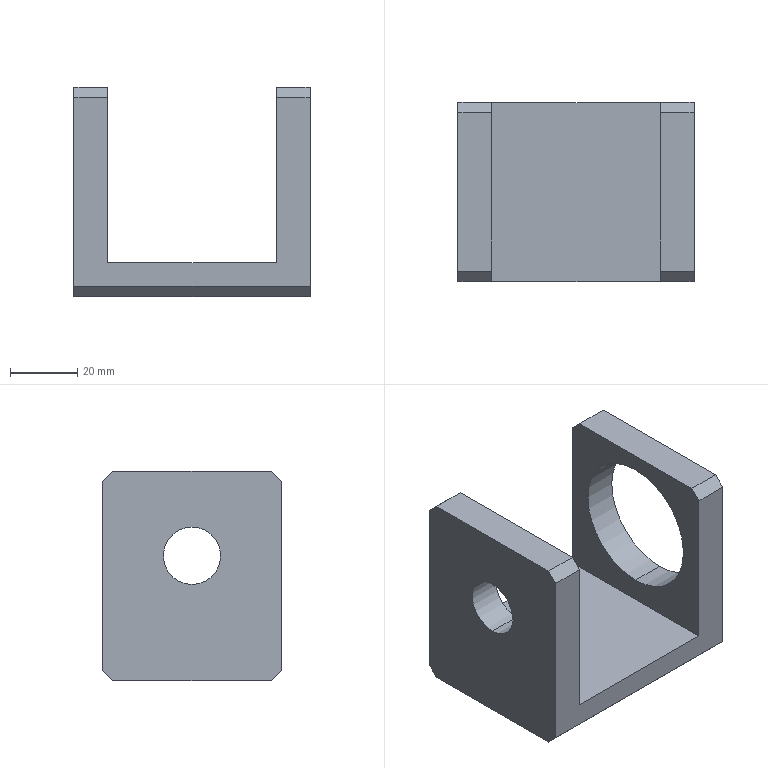Part | SolidWorks | features ICE 4, Chamfer 3, 3DProfileFeature 1, Extrusion 1, HoleWzd 1 | 1 solid | 20 faces | box 70 x 53 x 62 mm | volume 76574 mm3 | plane 16 | cylinder 4 | commonest cylinder face diameters 17 x2 40 x2
STEP:
#1=CARTESIAN_POINT('',(60.,0.,-5.));
#2=VERTEX_POINT('',#1);
#3=CARTESIAN_POINT('',(60.,0.,-45.));
#4=VERTEX_POINT('',#3);
#5=CARTESIAN_POINT('',(60.,0.,-25.));
#6=DIRECTION('',(1.,0.,0.));
#7=DIRECTION('',(0.,0.,1.));
#8=AXIS2_PLACEMENT_3D('',#5,#6,#7);
#9=CIRCLE('',#8,20.);
#10=EDGE_CURVE('',#2,#4,#9,.T.);
#11=ORIENTED_EDGE('',*,*,#10,.T.);
#12=CARTESIAN_POINT('',(50.,0.,-45.));
#13=VERTEX_POINT('',#12);
#14=CARTESIAN_POINT('',(60.001,0.,-45.));
#15=DIRECTION('',(-1.,0.,0.));
#16=VECTOR('',#15,1000.);
#17=LINE('',#14,#16);
#18=EDGE_CURVE('',#4,#13,#17,.T.);
#19=ORIENTED_EDGE('',*,*,#18,.T.);
#20=CARTESIAN_POINT('',(50.,0.,-5.));
#21=VERTEX_POINT('',#20);
#22=CARTESIAN_POINT('',(50.,0.,-25.));
#23=DIRECTION('',(-1.,0.,0.));
#24=DIRECTION('',(0.,0.,1.));
#25=AXIS2_PLACEMENT_3D('',#22,#23,#24);
#26=CIRCLE('',#25,20.);
#27=EDGE_CURVE('',#13,#21,#26,.T.);
#28=ORIENTED_EDGE('',*,*,#27,.T.);
#29=CARTESIAN_POINT('',(60.001,0.,-5.));
#30=DIRECTION('',(-1.,0.,0.));
#31=VECTOR('',#30,1000.);
#32=LINE('',#29,#31);
#33=EDGE_CURVE('',#2,#21,#32,.T.);
#34=ORIENTED_EDGE('',*,*,#33,.F.);
#35=EDGE_LOOP('',(#11,#19,#28,#34));
#36=FACE_OUTER_BOUND('',#35,.T.);
#37=CARTESIAN_POINT('',(60.001,0.,-25.));
#38=DIRECTION('',(-1.,0.,0.));
#39=DIRECTION('',(0.,0.,1.));
#40=AXIS2_PLACEMENT_3D('',#37,#38,#39);
#41=CYLINDRICAL_SURFACE('',#40,20.);
#42=ADVANCED_FACE('',(#36),#41,.F.);
#43=CARTESIAN_POINT('',(0.,0.,-16.5));
#44=VERTEX_POINT('',#43);
#45=CARTESIAN_POINT('',(0.,0.,-33.5));
#46=VERTEX_POINT('',#45);
#47=CARTESIAN_POINT('',(0.,0.,-25.));
#48=DIRECTION('',(1.,0.,0.));
#49=DIRECTION('',(0.,0.,1.));
#50=AXIS2_PLACEMENT_3D('',#47,#48,#49);
#51=CIRCLE('',#50,8.5);
#52=EDGE_CURVE('',#44,#46,#51,.T.);
#53=ORIENTED_EDGE('',*,*,#52,.T.);
#54=CARTESIAN_POINT('',(-10.,0.,-33.5));
#55=VERTEX_POINT('',#54);
#56=CARTESIAN_POINT('',(60.001,0.,-33.5));
#57=DIRECTION('',(-1.,0.,0.));
#58=VECTOR('',#57,1000.);
#59=LINE('',#56,#58);
#60=EDGE_CURVE('',#46,#55,#59,.T.);
#61=ORIENTED_EDGE('',*,*,#60,.T.);
#62=CARTESIAN_POINT('',(-10.,0.,-16.5));
#63=VERTEX_POINT('',#62);
#64=CARTESIAN_POINT('',(-10.,0.,-25.));
#65=DIRECTION('',(-1.,0.,0.));
#66=DIRECTION('',(0.,0.,1.));
#67=AXIS2_PLACEMENT_3D('',#64,#65,#66);
#68=CIRCLE('',#67,8.5);
#69=EDGE_CURVE('',#55,#63,#68,.T.);
#70=ORIENTED_EDGE('',*,*,#69,.T.);
#71=CARTESIAN_POINT('',(60.001,0.,-16.5));
#72=DIRECTION('',(-1.,0.,0.));
#73=VECTOR('',#72,1000.);
#74=LINE('',#71,#73);
#75=EDGE_CURVE('',#44,#63,#74,.T.);
#76=ORIENTED_EDGE('',*,*,#75,.F.);
#77=EDGE_LOOP('',(#53,#61,#70,#76));
#78=FACE_OUTER_BOUND('',#77,.T.);
#79=CARTESIAN_POINT('',(60.001,0.,-25.));
#80=DIRECTION('',(-1.,0.,0.));
#81=DIRECTION('',(0.,0.,1.));
#82=AXIS2_PLACEMENT_3D('',#79,#80,#81);
#83=CYLINDRICAL_SURFACE('',#82,8.5);
#84=ADVANCED_FACE('',(#78),#83,.F.);
#85=CARTESIAN_POINT('',(-10.,23.5,0.));
#86=VERTEX_POINT('',#85);
#87=CARTESIAN_POINT('',(-10.,-23.5,0.));
#88=VERTEX_POINT('',#87);
#89=CARTESIAN_POINT('',(-10.,26.5,0.));
#90=DIRECTION('',(0.,-1.,0.));
#91=VECTOR('',#90,1000.);
#92=LINE('',#89,#91);
#93=EDGE_CURVE('',#86,#88,#92,.T.);
#94=ORIENTED_EDGE('',*,*,#93,.T.);
#95=CARTESIAN_POINT('',(0.,-23.5,0.));
#96=VERTEX_POINT('',#95);
#97=CARTESIAN_POINT('',(0.,-23.5,0.));
#98=DIRECTION('',(1.,0.,0.));
#99=VECTOR('',#98,1000.);
#100=LINE('',#97,#99);
#101=EDGE_CURVE('',#88,#96,#100,.T.);
#102=ORIENTED_EDGE('',*,*,#101,.T.);
#103=CARTESIAN_POINT('',(0.,23.5,0.));
#104=VERTEX_POINT('',#103);
#105=CARTESIAN_POINT('',(0.,26.5,0.));
#106=DIRECTION('',(0.,-1.,0.));
#107=VECTOR('',#106,1000.);
#108=LINE('',#105,#107);
#109=EDGE_CURVE('',#104,#96,#108,.T.);
#110=ORIENTED_EDGE('',*,*,#109,.F.);
#111=CARTESIAN_POINT('',(0.,23.5,0.));
#112=DIRECTION('',(-1.,0.,0.));
#113=VECTOR('',#112,1000.);
#114=LINE('',#111,#113);
#115=EDGE_CURVE('',#104,#86,#114,.T.);
#116=ORIENTED_EDGE('',*,*,#115,.T.);
#117=EDGE_LOOP('',(#94,#102,#110,#116));
#118=FACE_OUTER_BOUND('',#117,.T.);
#119=CARTESIAN_POINT('',(0.,26.5,0.));
#120=DIRECTION('',(0.,0.,-1.));
#121=DIRECTION('',(-1.,0.,0.));
#122=AXIS2_PLACEMENT_3D('',#119,#120,#121);
#123=PLANE('',#122);
#124=ADVANCED_FACE('',(#118),#123,.F.);
#125=ORIENTED_EDGE('',*,*,#52,.F.);
#126=CARTESIAN_POINT('',(0.,0.,-25.));
#127=DIRECTION('',(1.,0.,0.));
#128=DIRECTION('',(0.,0.,1.));
#129=AXIS2_PLACEMENT_3D('',#126,#127,#128);
#130=CIRCLE('',#129,8.5);
#131=EDGE_CURVE('',#46,#44,#130,.T.);
#132=ORIENTED_EDGE('',*,*,#131,.F.);
#133=EDGE_LOOP('',(#125,#132));
#134=FACE_BOUND('',#133,.T.);
#135=ORIENTED_EDGE('',*,*,#109,.T.);
#136=CARTESIAN_POINT('',(0.,-26.5,-3.));
#137=VERTEX_POINT('',#136);
#138=CARTESIAN_POINT('',(0.,-23.5,0.));
#139=DIRECTION('',(0.,-0.7071,-0.7071));
#140=VECTOR('',#139,1000.);
#141=LINE('',#138,#140);
#142=EDGE_CURVE('',#96,#137,#141,.T.);
#143=ORIENTED_EDGE('',*,*,#142,.T.);
#144=CARTESIAN_POINT('',(0.,-26.5,-52.));
#145=VERTEX_POINT('',#144);
#146=CARTESIAN_POINT('',(0.,-26.5,0.));
#147=DIRECTION('',(0.,0.,-1.));
#148=VECTOR('',#147,1000.);
#149=LINE('',#146,#148);
#150=EDGE_CURVE('',#137,#145,#149,.T.);
#151=ORIENTED_EDGE('',*,*,#150,.T.);
#152=CARTESIAN_POINT('',(0.,26.5,-52.));
#153=VERTEX_POINT('',#152);
#154=CARTESIAN_POINT('',(0.,26.5,-52.));
#155=DIRECTION('',(0.,-1.,0.));
#156=VECTOR('',#155,1000.);
#157=LINE('',#154,#156);
#158=EDGE_CURVE('',#153,#145,#157,.T.);
#159=ORIENTED_EDGE('',*,*,#158,.F.);
#160=CARTESIAN_POINT('',(0.,26.5,-3.));
#161=VERTEX_POINT('',#160);
#162=CARTESIAN_POINT('',(0.,26.5,0.));
#163=DIRECTION('',(0.,0.,-1.));
#164=VECTOR('',#163,1000.);
#165=LINE('',#162,#164);
#166=EDGE_CURVE('',#161,#153,#165,.T.);
#167=ORIENTED_EDGE('',*,*,#166,.F.);
#168=CARTESIAN_POINT('',(0.,26.5,-3.));
#169=DIRECTION('',(0.,-0.7071,0.7071));
#170=VECTOR('',#169,1000.);
#171=LINE('',#168,#170);
#172=EDGE_CURVE('',#161,#104,#171,.T.);
#173=ORIENTED_EDGE('',*,*,#172,.T.);
#174=EDGE_LOOP('',(#135,#143,#151,#159,#167,#173));
#175=FACE_OUTER_BOUND('',#174,.T.);
#176=CARTESIAN_POINT('',(0.,26.5,0.));
#177=DIRECTION('',(-1.,0.,0.));
#178=DIRECTION('',(0.,0.,1.));
#179=AXIS2_PLACEMENT_3D('',#176,#177,#178);
#180=PLANE('',#179);
#181=ADVANCED_FACE('',(#134,#175),#180,.F.);
#182=CARTESIAN_POINT('',(50.,-26.5,-52.));
#183=VERTEX_POINT('',#182);
#184=CARTESIAN_POINT('',(0.,-26.5,-52.));
#185=DIRECTION('',(1.,0.,0.));
#186=VECTOR('',#185,1000.);
#187=LINE('',#184,#186);
#188=EDGE_CURVE('',#145,#183,#187,.T.);
#189=ORIENTED_EDGE('',*,*,#188,.T.);
#190=CARTESIAN_POINT('',(50.,26.5,-52.));
#191=VERTEX_POINT('',#190);
#192=CARTESIAN_POINT('',(50.,26.5,-52.));
#193=DIRECTION('',(0.,-1.,0.));
#194=VECTOR('',#193,1000.);
#195=LINE('',#192,#194);
#196=EDGE_CURVE('',#191,#183,#195,.T.);
#197=ORIENTED_EDGE('',*,*,#196,.F.);
#198=CARTESIAN_POINT('',(0.,26.5,-52.));
#199=DIRECTION('',(1.,0.,0.));
#200=VECTOR('',#199,1000.);
#201=LINE('',#198,#200);
#202=EDGE_CURVE('',#153,#191,#201,.T.);
#203=ORIENTED_EDGE('',*,*,#202,.F.);
#204=ORIENTED_EDGE('',*,*,#158,.T.);
#205=EDGE_LOOP('',(#189,#197,#203,#204));
#206=FACE_OUTER_BOUND('',#205,.T.);
#207=CARTESIAN_POINT('',(0.,26.5,-52.));
#208=DIRECTION('',(0.,0.,-1.));
#209=DIRECTION('',(-1.,0.,0.));
#210=AXIS2_PLACEMENT_3D('',#207,#208,#209);
#211=PLANE('',#210);
#212=ADVANCED_FACE('',(#206),#211,.F.);
#213=CARTESIAN_POINT('',(50.,0.,-25.));
#214=DIRECTION('',(-1.,0.,0.));
#215=DIRECTION('',(0.,0.,1.));
#216=AXIS2_PLACEMENT_3D('',#213,#214,#215);
#217=CIRCLE('',#216,20.);
#218=EDGE_CURVE('',#21,#13,#217,.T.);
#219=ORIENTED_EDGE('',*,*,#218,.F.);
#220=ORIENTED_EDGE('',*,*,#27,.F.);
#221=EDGE_LOOP('',(#219,#220));
#222=FACE_BOUND('',#221,.T.);
#223=CARTESIAN_POINT('',(50.,23.5,0.));
#224=VERTEX_POINT('',#223);
#225=CARTESIAN_POINT('',(50.,-23.5,0.));
#226=VERTEX_POINT('',#225);
#227=CARTESIAN_POINT('',(50.,26.5,0.));
#228=DIRECTION('',(0.,-1.,0.));
#229=VECTOR('',#228,1000.);
#230=LINE('',#227,#229);
#231=EDGE_CURVE('',#224,#226,#230,.T.);
#232=ORIENTED_EDGE('',*,*,#231,.F.);
#233=CARTESIAN_POINT('',(50.,26.5,-3.));
#234=VERTEX_POINT('',#233);
#235=CARTESIAN_POINT('',(50.,26.5,-3.));
#236=DIRECTION('',(0.,0.7071,-0.7071));
#237=VECTOR('',#236,1000.);
#238=LINE('',#235,#237);
#239=EDGE_CURVE('',#224,#234,#238,.T.);
#240=ORIENTED_EDGE('',*,*,#239,.T.);
#241=CARTESIAN_POINT('',(50.,26.5,-52.));
#242=DIRECTION('',(0.,0.,1.));
#243=VECTOR('',#242,1000.);
#244=LINE('',#241,#243);
#245=EDGE_CURVE('',#191,#234,#244,.T.);
#246=ORIENTED_EDGE('',*,*,#245,.F.);
#247=ORIENTED_EDGE('',*,*,#196,.T.);
#248=CARTESIAN_POINT('',(50.,-26.5,-3.));
#249=VERTEX_POINT('',#248);
#250=CARTESIAN_POINT('',(50.,-26.5,-52.));
#251=DIRECTION('',(0.,0.,1.));
#252=VECTOR('',#251,1000.);
#253=LINE('',#250,#252);
#254=EDGE_CURVE('',#183,#249,#253,.T.);
#255=ORIENTED_EDGE('',*,*,#254,.T.);
#256=CARTESIAN_POINT('',(50.,-23.5,0.));
#257=DIRECTION('',(0.,0.7071,0.7071));
#258=VECTOR('',#257,1000.);
#259=LINE('',#256,#258);
#260=EDGE_CURVE('',#249,#226,#259,.T.);
#261=ORIENTED_EDGE('',*,*,#260,.T.);
#262=EDGE_LOOP('',(#232,#240,#246,#247,#255,#261));
#263=FACE_OUTER_BOUND('',#262,.T.);
#264=CARTESIAN_POINT('',(50.,26.5,-52.));
#265=DIRECTION('',(1.,0.,0.));
#266=DIRECTION('',(0.,0.,-1.));
#267=AXIS2_PLACEMENT_3D('',#264,#265,#266);
#268=PLANE('',#267);
#269=ADVANCED_FACE('',(#222,#263),#268,.F.);
#270=CARTESIAN_POINT('',(60.,23.5,0.));
#271=VERTEX_POINT('',#270);
#272=CARTESIAN_POINT('',(60.,-23.5,0.));
#273=VERTEX_POINT('',#272);
#274=CARTESIAN_POINT('',(60.,26.5,0.));
#275=DIRECTION('',(0.,-1.,0.));
#276=VECTOR('',#275,1000.);
#277=LINE('',#274,#276);
#278=EDGE_CURVE('',#271,#273,#277,.T.);
#279=ORIENTED_EDGE('',*,*,#278,.F.);
#280=CARTESIAN_POINT('',(60.,23.5,0.));
#281=DIRECTION('',(-1.,0.,0.));
#282=VECTOR('',#281,1000.);
#283=LINE('',#280,#282);
#284=EDGE_CURVE('',#271,#224,#283,.T.);
#285=ORIENTED_EDGE('',*,*,#284,.T.);
#286=ORIENTED_EDGE('',*,*,#231,.T.);
#287=CARTESIAN_POINT('',(60.,-23.5,0.));
#288=DIRECTION('',(1.,0.,0.));
#289=VECTOR('',#288,1000.);
#290=LINE('',#287,#289);
#291=EDGE_CURVE('',#226,#273,#290,.T.);
#292=ORIENTED_EDGE('',*,*,#291,.T.);
#293=EDGE_LOOP('',(#279,#285,#286,#292));
#294=FACE_OUTER_BOUND('',#293,.T.);
#295=CARTESIAN_POINT('',(60.,26.5,0.));
#296=DIRECTION('',(0.,0.,-1.));
#297=DIRECTION('',(-1.,0.,0.));
#298=AXIS2_PLACEMENT_3D('',#295,#296,#297);
#299=PLANE('',#298);
#300=ADVANCED_FACE('',(#294),#299,.F.);
#301=ORIENTED_EDGE('',*,*,#10,.F.);
#302=CARTESIAN_POINT('',(60.,0.,-25.));
#303=DIRECTION('',(1.,0.,0.));
#304=DIRECTION('',(0.,0.,1.));
#305=AXIS2_PLACEMENT_3D('',#302,#303,#304);
#306=CIRCLE('',#305,20.);
#307=EDGE_CURVE('',#4,#2,#306,.T.);
#308=ORIENTED_EDGE('',*,*,#307,.F.);
#309=EDGE_LOOP('',(#301,#308));
#310=FACE_BOUND('',#309,.T.);
#311=CARTESIAN_POINT('',(60.,26.5,-3.));
#312=VERTEX_POINT('',#311);
#313=CARTESIAN_POINT('',(60.,26.5,-59.));
#314=VERTEX_POINT('',#313);
#315=CARTESIAN_POINT('',(60.,26.5,-62.));
#316=DIRECTION('',(0.,0.,-1.));
#317=VECTOR('',#316,1000.);
#318=LINE('',#315,#317);
#319=EDGE_CURVE('',#312,#314,#318,.T.);
#320=ORIENTED_EDGE('',*,*,#319,.F.);
#321=CARTESIAN_POINT('',(60.,26.5,-3.));
#322=DIRECTION('',(0.,-0.7071,0.7071));
#323=VECTOR('',#322,1000.);
#324=LINE('',#321,#323);
#325=EDGE_CURVE('',#312,#271,#324,.T.);
#326=ORIENTED_EDGE('',*,*,#325,.T.);
#327=ORIENTED_EDGE('',*,*,#278,.T.);
#328=CARTESIAN_POINT('',(60.,-26.5,-3.));
#329=VERTEX_POINT('',#328);
#330=CARTESIAN_POINT('',(60.,-23.5,0.));
#331=DIRECTION('',(0.,-0.7071,-0.7071));
#332=VECTOR('',#331,1000.);
#333=LINE('',#330,#332);
#334=EDGE_CURVE('',#273,#329,#333,.T.);
#335=ORIENTED_EDGE('',*,*,#334,.T.);
#336=CARTESIAN_POINT('',(60.,-26.5,-59.));
#337=VERTEX_POINT('',#336);
#338=CARTESIAN_POINT('',(60.,-26.5,-62.));
#339=DIRECTION('',(0.,0.,-1.));
#340=VECTOR('',#339,1000.);
#341=LINE('',#338,#340);
#342=EDGE_CURVE('',#329,#337,#341,.T.);
#343=ORIENTED_EDGE('',*,*,#342,.T.);
#344=CARTESIAN_POINT('',(60.,-23.5,-62.));
#345=VERTEX_POINT('',#344);
#346=CARTESIAN_POINT('',(60.,-23.5,-62.));
#347=DIRECTION('',(0.,0.7071,-0.7071));
#348=VECTOR('',#347,1000.);
#349=LINE('',#346,#348);
#350=EDGE_CURVE('',#337,#345,#349,.T.);
#351=ORIENTED_EDGE('',*,*,#350,.T.);
#352=CARTESIAN_POINT('',(60.,23.5,-62.));
#353=VERTEX_POINT('',#352);
#354=CARTESIAN_POINT('',(60.,26.5,-62.));
#355=DIRECTION('',(0.,-1.,0.));
#356=VECTOR('',#355,1000.);
#357=LINE('',#354,#356);
#358=EDGE_CURVE('',#353,#345,#357,.T.);
#359=ORIENTED_EDGE('',*,*,#358,.F.);
#360=CARTESIAN_POINT('',(60.,26.5,-59.));
#361=DIRECTION('',(0.,0.7071,0.7071));
#362=VECTOR('',#361,1000.);
#363=LINE('',#360,#362);
#364=EDGE_CURVE('',#353,#314,#363,.T.);
#365=ORIENTED_EDGE('',*,*,#364,.T.);
#366=EDGE_LOOP('',(#320,#326,#327,#335,#343,#351,#359,#365));
#367=FACE_OUTER_BOUND('',#366,.T.);
#368=CARTESIAN_POINT('',(60.,26.5,-62.));
#369=DIRECTION('',(-1.,0.,0.));
#370=DIRECTION('',(0.,0.,1.));
#371=AXIS2_PLACEMENT_3D('',#368,#369,#370);
#372=PLANE('',#371);
#373=ADVANCED_FACE('',(#310,#367),#372,.F.);
#374=CARTESIAN_POINT('',(-10.,23.5,-62.));
#375=VERTEX_POINT('',#374);
#376=CARTESIAN_POINT('',(-10.,-23.5,-62.));
#377=VERTEX_POINT('',#376);
#378=CARTESIAN_POINT('',(-10.,26.5,-62.));
#379=DIRECTION('',(0.,-1.,0.));
#380=VECTOR('',#379,1000.);
#381=LINE('',#378,#380);
#382=EDGE_CURVE('',#375,#377,#381,.T.);
#383=ORIENTED_EDGE('',*,*,#382,.F.);
#384=CARTESIAN_POINT('',(-10.,23.5,-62.));
#385=DIRECTION('',(1.,0.,0.));
#386=VECTOR('',#385,1000.);
#387=LINE('',#384,#386);
#388=EDGE_CURVE('',#375,#353,#387,.T.);
#389=ORIENTED_EDGE('',*,*,#388,.T.);
#390=ORIENTED_EDGE('',*,*,#358,.T.);
#391=CARTESIAN_POINT('',(-10.,-23.5,-62.));
#392=DIRECTION('',(-1.,0.,0.));
#393=VECTOR('',#392,1000.);
#394=LINE('',#391,#393);
#395=EDGE_CURVE('',#345,#377,#394,.T.);
#396=ORIENTED_EDGE('',*,*,#395,.T.);
#397=EDGE_LOOP('',(#383,#389,#390,#396));
#398=FACE_OUTER_BOUND('',#397,.T.);
#399=CARTESIAN_POINT('',(-10.,26.5,-62.));
#400=DIRECTION('',(0.,0.,1.));
#401=DIRECTION('',(1.,0.,0.));
#402=AXIS2_PLACEMENT_3D('',#399,#400,#401);
#403=PLANE('',#402);
#404=ADVANCED_FACE('',(#398),#403,.F.);
#405=CARTESIAN_POINT('',(-10.,0.,-25.));
#406=DIRECTION('',(-1.,0.,0.));
#407=DIRECTION('',(0.,0.,1.));
#408=AXIS2_PLACEMENT_3D('',#405,#406,#407);
#409=CIRCLE('',#408,8.5);
#410=EDGE_CURVE('',#63,#55,#409,.T.);
#411=ORIENTED_EDGE('',*,*,#410,.F.);
#412=ORIENTED_EDGE('',*,*,#69,.F.);
#413=EDGE_LOOP('',(#411,#412));
#414=FACE_BOUND('',#413,.T.);
#415=CARTESIAN_POINT('',(-10.,-26.5,-59.));
#416=VERTEX_POINT('',#415);
#417=CARTESIAN_POINT('',(-10.,-26.5,-3.));
#418=VERTEX_POINT('',#417);
#419=CARTESIAN_POINT('',(-10.,-26.5,0.));
#420=DIRECTION('',(0.,0.,1.));
#421=VECTOR('',#420,1000.);
#422=LINE('',#419,#421);
#423=EDGE_CURVE('',#416,#418,#422,.T.);
#424=ORIENTED_EDGE('',*,*,#423,.T.);
#425=CARTESIAN_POINT('',(-10.,-23.5,0.));
#426=DIRECTION('',(0.,0.7071,0.7071));
#427=VECTOR('',#426,1000.);
#428=LINE('',#425,#427);
#429=EDGE_CURVE('',#418,#88,#428,.T.);
#430=ORIENTED_EDGE('',*,*,#429,.T.);
#431=ORIENTED_EDGE('',*,*,#93,.F.);
#432=CARTESIAN_POINT('',(-10.,26.5,-3.));
#433=VERTEX_POINT('',#432);
#434=CARTESIAN_POINT('',(-10.,26.5,-3.));
#435=DIRECTION('',(0.,0.7071,-0.7071));
#436=VECTOR('',#435,1000.);
#437=LINE('',#434,#436);
#438=EDGE_CURVE('',#86,#433,#437,.T.);
#439=ORIENTED_EDGE('',*,*,#438,.T.);
#440=CARTESIAN_POINT('',(-10.,26.5,-59.));
#441=VERTEX_POINT('',#440);
#442=CARTESIAN_POINT('',(-10.,26.5,0.));
#443=DIRECTION('',(0.,0.,1.));
#444=VECTOR('',#443,1000.);
#445=LINE('',#442,#444);
#446=EDGE_CURVE('',#441,#433,#445,.T.);
#447=ORIENTED_EDGE('',*,*,#446,.F.);
#448=CARTESIAN_POINT('',(-10.,26.5,-59.));
#449=DIRECTION('',(0.,-0.7071,-0.7071));
#450=VECTOR('',#449,1000.);
#451=LINE('',#448,#450);
#452=EDGE_CURVE('',#441,#375,#451,.T.);
#453=ORIENTED_EDGE('',*,*,#452,.T.);
#454=ORIENTED_EDGE('',*,*,#382,.T.);
#455=CARTESIAN_POINT('',(-10.,-23.5,-62.));
#456=DIRECTION('',(0.,-0.7071,0.7071));
#457=VECTOR('',#456,1000.);
#458=LINE('',#455,#457);
#459=EDGE_CURVE('',#377,#416,#458,.T.);
#460=ORIENTED_EDGE('',*,*,#459,.T.);
#461=EDGE_LOOP('',(#424,#430,#431,#439,#447,#453,#454,#460));
#462=FACE_OUTER_BOUND('',#461,.T.);
#463=CARTESIAN_POINT('',(-10.,26.5,0.));
#464=DIRECTION('',(1.,0.,0.));
#465=DIRECTION('',(0.,0.,-1.));
#466=AXIS2_PLACEMENT_3D('',#463,#464,#465);
#467=PLANE('',#466);
#468=ADVANCED_FACE('',(#414,#462),#467,.F.);
#469=ORIENTED_EDGE('',*,*,#245,.T.);
#470=CARTESIAN_POINT('',(0.,26.5,-3.));
#471=DIRECTION('',(1.,0.,0.));
#472=VECTOR('',#471,1000.);
#473=LINE('',#470,#472);
#474=EDGE_CURVE('',#234,#312,#473,.T.);
#475=ORIENTED_EDGE('',*,*,#474,.T.);
#476=ORIENTED_EDGE('',*,*,#319,.T.);
#477=CARTESIAN_POINT('',(0.,26.5,-59.));
#478=DIRECTION('',(-1.,0.,0.));
#479=VECTOR('',#478,1000.);
#480=LINE('',#477,#479);
#481=EDGE_CURVE('',#314,#441,#480,.T.);
#482=ORIENTED_EDGE('',*,*,#481,.T.);
#483=ORIENTED_EDGE('',*,*,#446,.T.);
#484=CARTESIAN_POINT('',(0.,26.5,-3.));
#485=DIRECTION('',(1.,0.,0.));
#486=VECTOR('',#485,1000.);
#487=LINE('',#484,#486);
#488=EDGE_CURVE('',#433,#161,#487,.T.);
#489=ORIENTED_EDGE('',*,*,#488,.T.);
#490=ORIENTED_EDGE('',*,*,#166,.T.);
#491=ORIENTED_EDGE('',*,*,#202,.T.);
#492=EDGE_LOOP('',(#469,#475,#476,#482,#483,#489,#490,#491));
#493=FACE_OUTER_BOUND('',#492,.T.);
#494=CARTESIAN_POINT('',(0.,26.5,0.));
#495=DIRECTION('',(0.,-1.,0.));
#496=DIRECTION('',(0.,0.,-1.));
#497=AXIS2_PLACEMENT_3D('',#494,#495,#496);
#498=PLANE('',#497);
#499=ADVANCED_FACE('',(#493),#498,.F.);
#500=ORIENTED_EDGE('',*,*,#342,.F.);
#501=CARTESIAN_POINT('',(50.,-26.5,-3.));
#502=DIRECTION('',(-1.,0.,0.));
#503=VECTOR('',#502,1000.);
#504=LINE('',#501,#503);
#505=EDGE_CURVE('',#329,#249,#504,.T.);
#506=ORIENTED_EDGE('',*,*,#505,.T.);
#507=ORIENTED_EDGE('',*,*,#254,.F.);
#508=ORIENTED_EDGE('',*,*,#188,.F.);
#509=ORIENTED_EDGE('',*,*,#150,.F.);
#510=CARTESIAN_POINT('',(-10.,-26.5,-3.));
#511=DIRECTION('',(-1.,0.,0.));
#512=VECTOR('',#511,1000.);
#513=LINE('',#510,#512);
#514=EDGE_CURVE('',#137,#418,#513,.T.);
#515=ORIENTED_EDGE('',*,*,#514,.T.);
#516=ORIENTED_EDGE('',*,*,#423,.F.);
#517=CARTESIAN_POINT('',(60.,-26.5,-59.));
#518=DIRECTION('',(1.,0.,0.));
#519=VECTOR('',#518,1000.);
#520=LINE('',#517,#519);
#521=EDGE_CURVE('',#416,#337,#520,.T.);
#522=ORIENTED_EDGE('',*,*,#521,.T.);
#523=EDGE_LOOP('',(#500,#506,#507,#508,#509,#515,#516,#522));
#524=FACE_OUTER_BOUND('',#523,.T.);
#525=CARTESIAN_POINT('',(0.,-26.5,0.));
#526=DIRECTION('',(0.,-1.,0.));
#527=DIRECTION('',(0.,0.,-1.));
#528=AXIS2_PLACEMENT_3D('',#525,#526,#527);
#529=PLANE('',#528);
#530=ADVANCED_FACE('',(#524),#529,.T.);
#531=ORIENTED_EDGE('',*,*,#60,.F.);
#532=ORIENTED_EDGE('',*,*,#131,.T.);
#533=ORIENTED_EDGE('',*,*,#75,.T.);
#534=ORIENTED_EDGE('',*,*,#410,.T.);
#535=EDGE_LOOP('',(#531,#532,#533,#534));
#536=FACE_OUTER_BOUND('',#535,.T.);
#537=CARTESIAN_POINT('',(60.001,0.,-25.));
#538=DIRECTION('',(-1.,0.,0.));
#539=DIRECTION('',(0.,0.,1.));
#540=AXIS2_PLACEMENT_3D('',#537,#538,#539);
#541=CYLINDRICAL_SURFACE('',#540,8.5);
#542=ADVANCED_FACE('',(#536),#541,.F.);
#543=ORIENTED_EDGE('',*,*,#18,.F.);
#544=ORIENTED_EDGE('',*,*,#307,.T.);
#545=ORIENTED_EDGE('',*,*,#33,.T.);
#546=ORIENTED_EDGE('',*,*,#218,.T.);
#547=EDGE_LOOP('',(#543,#544,#545,#546));
#548=FACE_OUTER_BOUND('',#547,.T.);
#549=CARTESIAN_POINT('',(60.001,0.,-25.));
#550=DIRECTION('',(-1.,0.,0.));
#551=DIRECTION('',(0.,0.,1.));
#552=AXIS2_PLACEMENT_3D('',#549,#550,#551);
#553=CYLINDRICAL_SURFACE('',#552,20.);
#554=ADVANCED_FACE('',(#548),#553,.F.);
#555=ORIENTED_EDGE('',*,*,#364,.F.);
#556=ORIENTED_EDGE('',*,*,#388,.F.);
#557=ORIENTED_EDGE('',*,*,#452,.F.);
#558=ORIENTED_EDGE('',*,*,#481,.F.);
#559=EDGE_LOOP('',(#555,#556,#557,#558));
#560=FACE_OUTER_BOUND('',#559,.T.);
#561=CARTESIAN_POINT('',(0.,26.5,-59.));
#562=DIRECTION('',(0.,-0.7071,0.7071));
#563=DIRECTION('',(-1.,0.,0.));
#564=AXIS2_PLACEMENT_3D('',#561,#562,#563);
#565=PLANE('',#564);
#566=ADVANCED_FACE('',(#560),#565,.F.);
#567=ORIENTED_EDGE('',*,*,#350,.F.);
#568=ORIENTED_EDGE('',*,*,#521,.F.);
#569=ORIENTED_EDGE('',*,*,#459,.F.);
#570=ORIENTED_EDGE('',*,*,#395,.F.);
#571=EDGE_LOOP('',(#567,#568,#569,#570));
#572=FACE_OUTER_BOUND('',#571,.T.);
#573=CARTESIAN_POINT('',(-10.,-23.5,-62.));
#574=DIRECTION('',(0.,-0.7071,-0.7071));
#575=DIRECTION('',(1.,0.,0.));
#576=AXIS2_PLACEMENT_3D('',#573,#574,#575);
#577=PLANE('',#576);
#578=ADVANCED_FACE('',(#572),#577,.T.);
#579=ORIENTED_EDGE('',*,*,#239,.F.);
#580=ORIENTED_EDGE('',*,*,#284,.F.);
#581=ORIENTED_EDGE('',*,*,#325,.F.);
#582=ORIENTED_EDGE('',*,*,#474,.F.);
#583=EDGE_LOOP('',(#579,#580,#581,#582));
#584=FACE_OUTER_BOUND('',#583,.T.);
#585=CARTESIAN_POINT('',(0.,26.5,-3.));
#586=DIRECTION('',(0.,-0.7071,-0.7071));
#587=DIRECTION('',(1.,0.,0.));
#588=AXIS2_PLACEMENT_3D('',#585,#586,#587);
#589=PLANE('',#588);
#590=ADVANCED_FACE('',(#584),#589,.F.);
#591=ORIENTED_EDGE('',*,*,#260,.F.);
#592=ORIENTED_EDGE('',*,*,#505,.F.);
#593=ORIENTED_EDGE('',*,*,#334,.F.);
#594=ORIENTED_EDGE('',*,*,#291,.F.);
#595=EDGE_LOOP('',(#591,#592,#593,#594));
#596=FACE_OUTER_BOUND('',#595,.T.);
#597=CARTESIAN_POINT('',(60.,-23.5,0.));
#598=DIRECTION('',(0.,-0.7071,0.7071));
#599=DIRECTION('',(-1.,0.,0.));
#600=AXIS2_PLACEMENT_3D('',#597,#598,#599);
#601=PLANE('',#600);
#602=ADVANCED_FACE('',(#596),#601,.T.);
#603=ORIENTED_EDGE('',*,*,#429,.F.);
#604=ORIENTED_EDGE('',*,*,#514,.F.);
#605=ORIENTED_EDGE('',*,*,#142,.F.);
#606=ORIENTED_EDGE('',*,*,#101,.F.);
#607=EDGE_LOOP('',(#603,#604,#605,#606));
#608=FACE_OUTER_BOUND('',#607,.T.);
#609=CARTESIAN_POINT('',(0.,-23.5,0.));
#610=DIRECTION('',(0.,-0.7071,0.7071));
#611=DIRECTION('',(-1.,0.,0.));
#612=AXIS2_PLACEMENT_3D('',#609,#610,#611);
#613=PLANE('',#612);
#614=ADVANCED_FACE('',(#608),#613,.T.);
#615=ORIENTED_EDGE('',*,*,#438,.F.);
#616=ORIENTED_EDGE('',*,*,#115,.F.);
#617=ORIENTED_EDGE('',*,*,#172,.F.);
#618=ORIENTED_EDGE('',*,*,#488,.F.);
#619=EDGE_LOOP('',(#615,#616,#617,#618));
#620=FACE_OUTER_BOUND('',#619,.T.);
#621=CARTESIAN_POINT('',(0.,26.5,-3.));
#622=DIRECTION('',(0.,-0.7071,-0.7071));
#623=DIRECTION('',(1.,0.,0.));
#624=AXIS2_PLACEMENT_3D('',#621,#622,#623);
#625=PLANE('',#624);
#626=ADVANCED_FACE('',(#620),#625,.F.);
#627=CLOSED_SHELL('',(#42,#84,#124,#181,#212,#269,#300,#373,#404,#468,#499,#530,#542,#554,#566,#578,#590,#602,#614,#626));
#628=MANIFOLD_SOLID_BREP('',#627);
#629=CARTESIAN_POINT('',(0.,0.,0.));
#630=DIRECTION('',(0.,0.,1.));
#631=DIRECTION('',(1.,0.,0.));
#632=AXIS2_PLACEMENT_3D('',#629,#630,#631);
#633=(LENGTH_UNIT()NAMED_UNIT(*)SI_UNIT(.MILLI.,.METRE.));
#634=UNCERTAINTY_MEASURE_WITH_UNIT(LENGTH_MEASURE(0.00001),#633,'','');
#635=(NAMED_UNIT(*)PLANE_ANGLE_UNIT()SI_UNIT($,.RADIAN.));
#636=(NAMED_UNIT(*)SI_UNIT($,.STERADIAN.)SOLID_ANGLE_UNIT());
#637=(GEOMETRIC_REPRESENTATION_CONTEXT(3)GLOBAL_UNCERTAINTY_ASSIGNED_CONTEXT((#634))GLOBAL_UNIT_ASSIGNED_CONTEXT((#633,#635,#636))REPRESENTATION_CONTEXT('',''));
#638=ADVANCED_BREP_SHAPE_REPRESENTATION('',(#628,#632),#637);